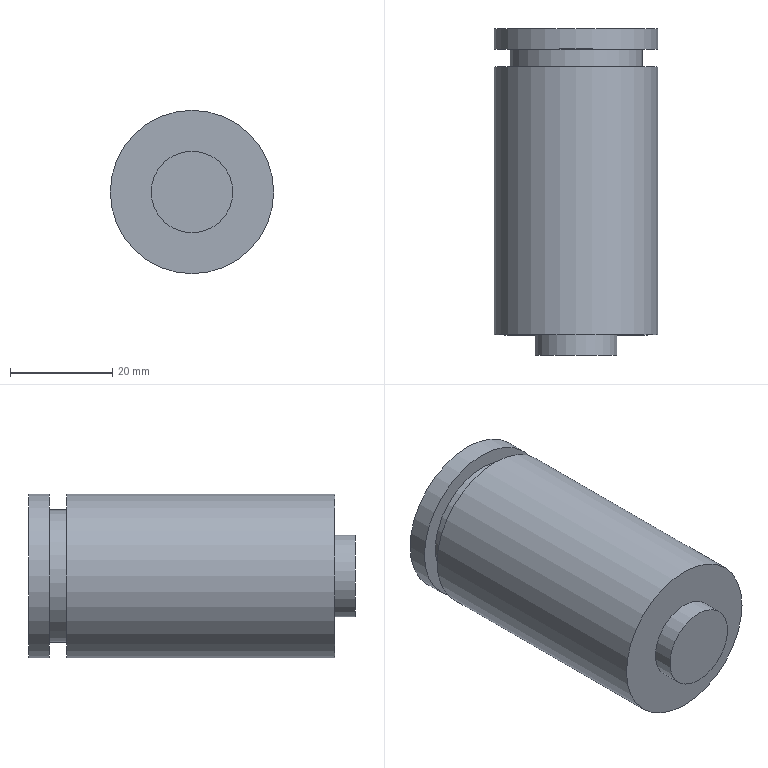Part | NX | features solid 2 | 1 solid | 9 faces | box 32 x 64 x 32 mm | volume 48102 mm3 | plane 5 | cylinder 4 | commonest cylinder face diameters 32 x2 16 x1 26 x1
STEP:
#1=CARTESIAN_POINT('',(713.,841.5,-185.));
#2=VERTEX_POINT('',#1);
#3=CARTESIAN_POINT('',(700.,841.5,-185.));
#4=DIRECTION('',(0.,-1.,0.));
#5=DIRECTION('',(1.,0.,0.));
#6=AXIS2_PLACEMENT_3D('',#3,#4,#5);
#7=CIRCLE('',#6,13.);
#8=EDGE_CURVE('',#2,#2,#7,.T.);
#9=ORIENTED_EDGE('',*,*,#8,.F.);
#10=EDGE_LOOP('',(#9));
#11=FACE_BOUND('',#10,.T.);
#12=CARTESIAN_POINT('',(713.,845.,-185.));
#13=VERTEX_POINT('',#12);
#14=CARTESIAN_POINT('',(700.,845.,-185.));
#15=DIRECTION('',(0.,-1.,0.));
#16=DIRECTION('',(1.,0.,0.));
#17=AXIS2_PLACEMENT_3D('',#14,#15,#16);
#18=CIRCLE('',#17,13.);
#19=EDGE_CURVE('',#13,#13,#18,.T.);
#20=ORIENTED_EDGE('',*,*,#19,.T.);
#21=EDGE_LOOP('',(#20));
#22=FACE_BOUND('',#21,.T.);
#23=CARTESIAN_POINT('',(700.,789.,-185.));
#24=DIRECTION('',(0.,1.,0.));
#25=DIRECTION('',(0.,0.,1.));
#26=AXIS2_PLACEMENT_3D('',#23,#24,#25);
#27=CYLINDRICAL_SURFACE('',#26,13.);
#28=ADVANCED_FACE('',(#11,#22),#27,.T.);
#29=CARTESIAN_POINT('',(716.,841.5,-185.));
#30=VERTEX_POINT('',#29);
#31=CARTESIAN_POINT('',(700.,841.5,-185.));
#32=DIRECTION('',(0.,-1.,0.));
#33=DIRECTION('',(1.,0.,0.));
#34=AXIS2_PLACEMENT_3D('',#31,#32,#33);
#35=CIRCLE('',#34,16.);
#36=EDGE_CURVE('',#30,#30,#35,.T.);
#37=ORIENTED_EDGE('',*,*,#36,.F.);
#38=EDGE_LOOP('',(#37));
#39=FACE_BOUND('',#38,.T.);
#40=ORIENTED_EDGE('',*,*,#8,.T.);
#41=EDGE_LOOP('',(#40));
#42=FACE_BOUND('',#41,.T.);
#43=CARTESIAN_POINT('',(700.,841.5,-172.));
#44=DIRECTION('',(0.,1.,0.));
#45=DIRECTION('',(0.,0.,1.));
#46=AXIS2_PLACEMENT_3D('',#43,#44,#45);
#47=PLANE('',#46);
#48=ADVANCED_FACE('',(#39,#42),#47,.T.);
#49=CARTESIAN_POINT('',(700.,789.,-169.));
#50=VERTEX_POINT('',#49);
#51=CARTESIAN_POINT('',(700.,789.,-185.));
#52=DIRECTION('',(0.,-1.,0.));
#53=DIRECTION('',(0.,0.,1.));
#54=AXIS2_PLACEMENT_3D('',#51,#52,#53);
#55=CIRCLE('',#54,16.);
#56=EDGE_CURVE('',#50,#50,#55,.T.);
#57=ORIENTED_EDGE('',*,*,#56,.F.);
#58=EDGE_LOOP('',(#57));
#59=FACE_BOUND('',#58,.T.);
#60=ORIENTED_EDGE('',*,*,#36,.T.);
#61=EDGE_LOOP('',(#60));
#62=FACE_BOUND('',#61,.T.);
#63=CARTESIAN_POINT('',(700.,789.,-185.));
#64=DIRECTION('',(0.,1.,0.));
#65=DIRECTION('',(0.,0.,1.));
#66=AXIS2_PLACEMENT_3D('',#63,#64,#65);
#67=CYLINDRICAL_SURFACE('',#66,16.);
#68=ADVANCED_FACE('',(#59,#62),#67,.T.);
#69=CARTESIAN_POINT('',(700.,789.,-177.));
#70=VERTEX_POINT('',#69);
#71=CARTESIAN_POINT('',(700.,789.,-185.));
#72=DIRECTION('',(0.,-1.,0.));
#73=DIRECTION('',(0.,0.,1.));
#74=AXIS2_PLACEMENT_3D('',#71,#72,#73);
#75=CIRCLE('',#74,8.);
#76=EDGE_CURVE('',#70,#70,#75,.T.);
#77=ORIENTED_EDGE('',*,*,#76,.F.);
#78=EDGE_LOOP('',(#77));
#79=FACE_BOUND('',#78,.T.);
#80=ORIENTED_EDGE('',*,*,#56,.T.);
#81=EDGE_LOOP('',(#80));
#82=FACE_BOUND('',#81,.T.);
#83=CARTESIAN_POINT('',(700.,789.,-201.));
#84=DIRECTION('',(0.,1.,0.));
#85=DIRECTION('',(0.,0.,1.));
#86=AXIS2_PLACEMENT_3D('',#83,#84,#85);
#87=PLANE('',#86);
#88=ADVANCED_FACE('',(#79,#82),#87,.F.);
#89=CARTESIAN_POINT('',(700.,849.,-169.));
#90=VERTEX_POINT('',#89);
#91=CARTESIAN_POINT('',(700.,849.,-185.));
#92=DIRECTION('',(0.,-1.,0.));
#93=DIRECTION('',(0.,0.,1.));
#94=AXIS2_PLACEMENT_3D('',#91,#92,#93);
#95=CIRCLE('',#94,16.);
#96=EDGE_CURVE('',#90,#90,#95,.T.);
#97=ORIENTED_EDGE('',*,*,#96,.F.);
#98=EDGE_LOOP('',(#97));
#99=FACE_BOUND('',#98,.T.);
#100=CARTESIAN_POINT('',(700.,849.,-215.));
#101=DIRECTION('',(0.,1.,0.));
#102=DIRECTION('',(0.,0.,1.));
#103=AXIS2_PLACEMENT_3D('',#100,#101,#102);
#104=PLANE('',#103);
#105=ADVANCED_FACE('',(#99),#104,.T.);
#106=CARTESIAN_POINT('',(716.,845.,-185.));
#107=VERTEX_POINT('',#106);
#108=CARTESIAN_POINT('',(700.,845.,-185.));
#109=DIRECTION('',(0.,-1.,0.));
#110=DIRECTION('',(1.,0.,0.));
#111=AXIS2_PLACEMENT_3D('',#108,#109,#110);
#112=CIRCLE('',#111,16.);
#113=EDGE_CURVE('',#107,#107,#112,.T.);
#114=ORIENTED_EDGE('',*,*,#113,.F.);
#115=EDGE_LOOP('',(#114));
#116=FACE_BOUND('',#115,.T.);
#117=ORIENTED_EDGE('',*,*,#96,.T.);
#118=EDGE_LOOP('',(#117));
#119=FACE_BOUND('',#118,.T.);
#120=CARTESIAN_POINT('',(700.,789.,-185.));
#121=DIRECTION('',(0.,1.,0.));
#122=DIRECTION('',(0.,0.,1.));
#123=AXIS2_PLACEMENT_3D('',#120,#121,#122);
#124=CYLINDRICAL_SURFACE('',#123,16.);
#125=ADVANCED_FACE('',(#116,#119),#124,.T.);
#126=ORIENTED_EDGE('',*,*,#113,.T.);
#127=EDGE_LOOP('',(#126));
#128=FACE_BOUND('',#127,.T.);
#129=ORIENTED_EDGE('',*,*,#19,.F.);
#130=EDGE_LOOP('',(#129));
#131=FACE_BOUND('',#130,.T.);
#132=CARTESIAN_POINT('',(700.,845.,-172.));
#133=DIRECTION('',(0.,1.,0.));
#134=DIRECTION('',(0.,0.,1.));
#135=AXIS2_PLACEMENT_3D('',#132,#133,#134);
#136=PLANE('',#135);
#137=ADVANCED_FACE('',(#128,#131),#136,.F.);
#138=CARTESIAN_POINT('',(700.,785.,-177.));
#139=VERTEX_POINT('',#138);
#140=CARTESIAN_POINT('',(700.,785.,-185.));
#141=DIRECTION('',(0.,-1.,0.));
#142=DIRECTION('',(0.,0.,1.));
#143=AXIS2_PLACEMENT_3D('',#140,#141,#142);
#144=CIRCLE('',#143,8.);
#145=EDGE_CURVE('',#139,#139,#144,.T.);
#146=ORIENTED_EDGE('',*,*,#145,.F.);
#147=EDGE_LOOP('',(#146));
#148=FACE_BOUND('',#147,.T.);
#149=ORIENTED_EDGE('',*,*,#76,.T.);
#150=EDGE_LOOP('',(#149));
#151=FACE_BOUND('',#150,.T.);
#152=CARTESIAN_POINT('',(700.,785.,-185.));
#153=DIRECTION('',(0.,1.,0.));
#154=DIRECTION('',(0.,0.,1.));
#155=AXIS2_PLACEMENT_3D('',#152,#153,#154);
#156=CYLINDRICAL_SURFACE('',#155,8.);
#157=ADVANCED_FACE('',(#148,#151),#156,.T.);
#158=ORIENTED_EDGE('',*,*,#145,.T.);
#159=EDGE_LOOP('',(#158));
#160=FACE_BOUND('',#159,.T.);
#161=CARTESIAN_POINT('',(700.,785.,-193.));
#162=DIRECTION('',(0.,1.,0.));
#163=DIRECTION('',(0.,0.,1.));
#164=AXIS2_PLACEMENT_3D('',#161,#162,#163);
#165=PLANE('',#164);
#166=ADVANCED_FACE('',(#160),#165,.F.);
#167=CLOSED_SHELL('',(#28,#48,#68,#88,#105,#125,#137,#157,#166));
#168=MANIFOLD_SOLID_BREP('',#167);
#169=(LENGTH_UNIT()NAMED_UNIT(*)SI_UNIT(.MILLI.,.METRE.));
#170=UNCERTAINTY_MEASURE_WITH_UNIT(LENGTH_MEASURE(0.00001),#169,'','');
#171=(NAMED_UNIT(*)PLANE_ANGLE_UNIT()SI_UNIT($,.RADIAN.));
#172=(NAMED_UNIT(*)SI_UNIT($,.STERADIAN.)SOLID_ANGLE_UNIT());
#173=(GEOMETRIC_REPRESENTATION_CONTEXT(3)GLOBAL_UNCERTAINTY_ASSIGNED_CONTEXT((#170))GLOBAL_UNIT_ASSIGNED_CONTEXT((#169,#171,#172))REPRESENTATION_CONTEXT('',''));
#174=ADVANCED_BREP_SHAPE_REPRESENTATION('',(#168),#173);